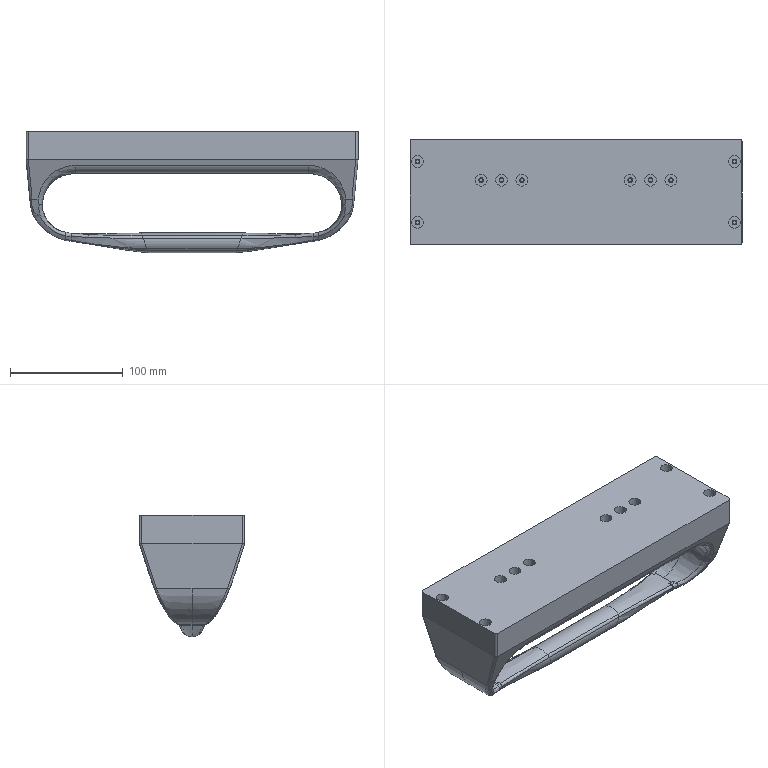NC program | NX | posted with a generic post | part box 294.078 x 93.5 x 107.5 mm
Lines 44852 to 45093 of 236164:
(ZLEVEL_PROFILE_COPY_COPY_1_COPY_COPY_COPY_COPY_1_COPY_COPY , TOOL : D10JING)
N89702 T11 M6
N89704 G54
N89706 G17 G0 G90 X-153.539 Y-4.502 B0. C0. S7500 M3
N89708 G43 Z30. H11
N89710 Z-12.917
N89712 G94 G1 Z-15.917 F1000.
N89714 X-153.119 Y-4.31
N89716 G3 X-152.539 Y-3.496 R1.
N89718 G1 X-151.833 Y3.889
N89720 X-148.185 Y41.977
N89722 G2 X-145.272 Y52.36 R34.864
N89724 X-139.337 Y61.783 R41.643
N89726 X-126.832 Y72.416 R48.33
N89728 X-113.846 Y77.75 R47.288
N89730 X-110.27 Y78.443 R37.8
N89732 G1 X-107.852 Y78.802
N89734 G3 X-84.406 Y82.587 R3032.247
N89736 G2 X-61.691 Y86.214 R2291.712
N89738 X-51.157 Y87.755 R643.354
N89740 X-43.04 Y88.725 R226.855
N89742 X-38.958 Y89. R60.732
N89744 G1 X39.042
N89746 G2 X43.766 Y88.661 R61.775
N89748 X55.845 Y87.105 R301.792
N89750 X78.637 Y83.541 R1576.826
N89752 G1 X96.91 Y80.554
N89754 X98.697 Y80.269
N89756 X107.918 Y78.805
N89758 X110.357 Y78.443
N89760 G2 X117.9 Y76.592 R42.136
N89762 X138.287 Y63.051 R48.687
N89764 X144.249 Y54.5 R43.068
N89766 X147.651 Y45.233 R36.517
N89768 X148.185 Y41.977 R30.69
N89770 G1 X151.833 Y3.889
N89772 X152.537 Y-3.489
N89774 G3 X153.118 Y-4.303 R1.
N89776 G1 X153.538 Y-4.495
N89778 Z-12.917
N89780 G0 Z30.
N89782 X-153.539 Y-4.502
N89784 Z-28.833
N89786 G1 Z-31.833
N89788 X-153.12 Y-4.31
N89790 G3 X-152.539 Y-3.495 R1.
N89792 G1 X-151.833 Y3.889
N89794 X-148.185 Y41.977
N89796 G2 X-145.273 Y52.36 R34.847
N89798 X-139.337 Y61.784 R41.736
N89800 X-126.832 Y72.416 R48.337
N89802 X-113.847 Y77.75 R47.257
N89804 X-110.27 Y78.443 R37.039
N89806 G1 X-107.852 Y78.802
N89808 G3 X-84.406 Y82.588 R3089.533
N89810 G2 X-61.183 Y86.292 R2238.47
N89812 X-50.278 Y87.873 R560.452
N89814 X-42.984 Y88.732 R215.014
N89816 X-38.958 Y89. R60.15
N89818 G1 X39.042
N89820 G2 X43.766 Y88.662 R61.191
N89822 X55.846 Y87.105 R300.842
N89824 X79.047 Y83.474 R1533.084
N89826 G1 X97.804 Y80.412
N89828 X99.143 Y80.197
N89830 X107.918 Y78.805
N89832 X110.357 Y78.443
N89834 G2 X117.9 Y76.593 R42.031
N89836 X138.287 Y63.051 R48.691
N89838 X144.435 Y54.142 R42.828
N89840 X147.822 Y44.391 R36.061
N89842 X148.185 Y41.977 R36.031
N89844 G1 X151.833 Y3.889
N89846 X152.538 Y-3.489
N89848 G3 X153.118 Y-4.303 R1.
N89850 G1 X153.539 Y-4.495
N89852 Z-28.833
N89854 G0 Z30.
N89856 X-153.54 Y-4.501
N89858 Z-44.75
N89860 G1 Z-47.75
N89862 X-153.121 Y-4.31
N89864 G3 X-152.54 Y-3.495 R1.
N89866 G1 X-151.833 Y3.889
N89868 X-148.185 Y41.977
N89870 G2 X-145.473 Y51.914 R34.66
N89872 X-139.759 Y61.269 R41.395
N89874 X-128.172 Y71.592 R48.076
N89876 X-115.221 Y77.395 R47.778
N89878 X-110.266 Y78.444 R39.039
N89880 G1 X-107.866 Y78.8
N89882 G3 X-82.173 Y82.953 R3566.777
N89884 G2 X-56.717 Y86.965 R1800.462
N89886 X-43.766 Y88.653 R301.443
N89888 X-38.958 Y89. R62.804
N89890 G1 X39.042
N89892 G2 X43.766 Y88.662 R60.198
N89894 X54.484 Y87.303 R283.501
N89896 X72.795 Y84.487 R1276.783
N89898 X91.354 Y81.464 R6633.224
N89900 G3 X107.918 Y78.805 R2243.827
N89902 G1 X110.35 Y78.444
N89904 G2 X117.454 Y76.743 R41.399
N89906 X138.444 Y62.875 R48.648
N89908 X144.435 Y54.142 R42.821
N89910 X147.822 Y44.392 R36.051
N89912 X148.185 Y41.977 R35.131
N89914 G1 X151.833 Y3.889
N89916 X152.538 Y-3.489
N89918 G3 X153.119 Y-4.303 R1.
N89920 G1 X153.539 Y-4.495
N89922 Z-44.75
N89924 G0 Z30.
(ZLEVEL_PROFILE_COPY_COPY_1_COPY_COPY_COPY_COPY_1_COPY_1 , TOOL : D10JING)
N89926 X109.794 Y60.443
N89928 Z-12.917
N89930 G1 Z-15.917
N89932 X109.526 Y60.999
N89934 G3 X108.699 Y61.563 R1.
N89936 G1 X108.252 Y61.596
N89938 G3 X98.863 Y62.029 R181.893
N89940 X84.518 Y62.16 R522.68
N89942 X66.509 Y61.962 R1407.439
N89944 X45.212 Y61.504 R2587.787
N89946 G1 X-45.102
N89948 G3 X-71.928 Y62.045 R2282.361
N89950 G1 X-73.269 Y62.06
N89952 X-73.716 Y62.067
N89954 G3 X-88.47 Y62.16 R894.341
N89956 X-99.648 Y62.008 R466.35
N89958 X-108.59 Y61.564 R171.161
N89960 X-116.19 Y59.394 R19.266
N89962 X-125.476 Y50.191 R22.337
N89964 X-127.3 Y45.271 R19.142
N89966 X-127.673 Y41.914 R15.801
N89968 G1 Y41.703
N89970 G3 X-124.015 Y29.417 R21.99
N89972 X-115.743 Y21.763 R23.877
N89974 X-103.167 Y18.5 R25.751
N89976 G1 X103.263
N89978 G3 X116.747 Y22.298 R25.688
N89980 X124.571 Y30.146 R23.707
N89982 X127.769 Y41.703 R21.973
N89984 G1 X127.768 Y41.883
N89986 G3 X126.912 Y47.056 R16.763
N89988 X123.9 Y52.839 R20.62
N89990 G1 X123.874 Y52.872
N89992 X123.539 Y53.318
N89994 G3 X116.747 Y59.146 R22.43
N89996 G1 X116.3 Y59.387
N89998 G3 X108.699 Y61.563 R19.256
N90000 X107.799 Y61.126 R1.
N90002 G1 X107.475 Y60.648
N90004 Z-12.917
N90006 G0 Z30.
N90008 X109.794 Y60.443
N90010 Z-28.833
N90012 G1 Z-31.833
N90014 X109.526 Y60.999
N90016 G3 X108.699 Y61.563 R1.
N90018 G1 X108.252 Y61.596
N90020 G3 X98.863 Y62.029 R181.9
N90022 X84.518 Y62.16 R522.68
N90024 X66.509 Y61.962 R1407.444
N90026 X45.212 Y61.504 R2587.787
N90028 G1 X-45.102
N90030 G3 X-71.928 Y62.045 R2282.361
N90032 G1 X-73.269 Y62.06
N90034 X-73.716 Y62.067
N90036 G3 X-88.47 Y62.16 R894.341
N90038 X-99.648 Y62.008 R466.35
N90040 X-108.59 Y61.564 R171.15
N90042 X-116.19 Y59.394 R19.266
N90044 X-125.476 Y50.191 R22.337
N90046 X-127.3 Y45.271 R19.142
N90048 X-127.673 Y41.913 R15.8
N90050 G1 Y41.703
N90052 G3 X-124.015 Y29.417 R21.997
N90054 X-115.743 Y21.763 R23.876
N90056 X-103.167 Y18.5 R25.759
N90058 G1 X103.257
N90060 G3 X116.3 Y22.028 R25.713
N90062 X124.571 Y30.147 R23.759
N90064 X127.769 Y41.703 R21.975
N90066 G1 X127.768 Y41.876
N90068 G3 X126.912 Y47.054 R16.758
N90070 X123.9 Y52.839 R20.62
N90072 G1 X123.874 Y52.872
N90074 X123.539 Y53.318
N90076 G3 X116.747 Y59.146 R22.43
N90078 G1 X116.3 Y59.387
N90080 G3 X108.699 Y61.563 R19.256
N90082 X107.799 Y61.126 R1.
N90084 G1 X107.475 Y60.648
N90086 Z-28.833
N90088 G0 Z30.
N90090 X109.794 Y60.443
N90092 Z-44.75
N90094 G1 Z-47.75
N90096 X109.526 Y60.999
N90098 G3 X108.699 Y61.563 R1.
N90100 G1 X108.252 Y61.596
N90102 G3 X98.863 Y62.029 R181.908
N90104 X84.518 Y62.16 R522.68
N90106 X66.509 Y61.962 R1407.448
N90108 X45.212 Y61.504 R2587.787
N90110 G1 X-45.102
N90112 G3 X-71.928 Y62.044 R2282.361
N90114 G1 X-73.269 Y62.06
N90116 X-73.716 Y62.067
N90118 G3 X-88.47 Y62.16 R894.341
N90120 X-99.648 Y62.008 R466.35
N90122 X-108.59 Y61.564 R171.138
N90124 X-116.19 Y59.394 R19.266
N90126 X-125.476 Y50.191 R22.337
N90128 X-127.3 Y45.271 R19.142
N90130 X-127.673 Y41.913 R15.8
N90132 G1 Y41.703
N90134 G3 X-124.015 Y29.417 R21.997
N90136 X-115.743 Y21.763 R23.876
N90138 X-103.167 Y18.5 R25.759
N90140 G1 X103.257
N90142 G3 X116.3 Y22.028 R25.713
N90144 X124.571 Y30.147 R23.759
N90146 X127.769 Y41.703 R21.975
N90148 G1 X127.768 Y41.876
N90150 G3 X126.912 Y47.054 R16.758
N90152 X123.9 Y52.839 R20.62
N90154 G1 X123.874 Y52.872
N90156 X123.539 Y53.318
N90158 G3 X116.747 Y59.146 R22.43
N90160 G1 X116.3 Y59.387
N90162 G3 X108.699 Y61.563 R19.256
N90164 X107.799 Y61.126 R1.
N90166 G1 X107.475 Y60.648
N90168 Z-44.75
N90170 G0 Z30.
N90172 M5